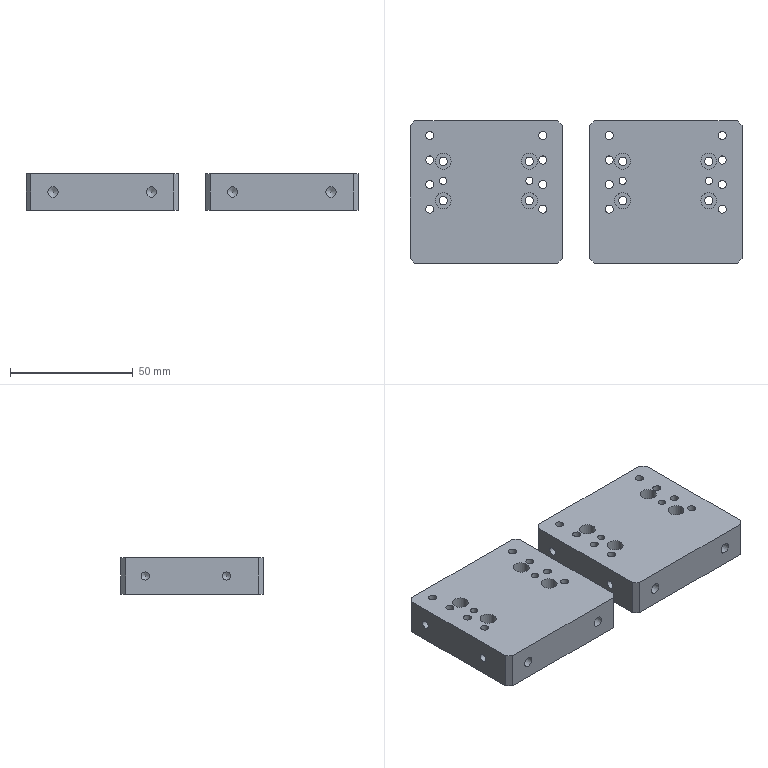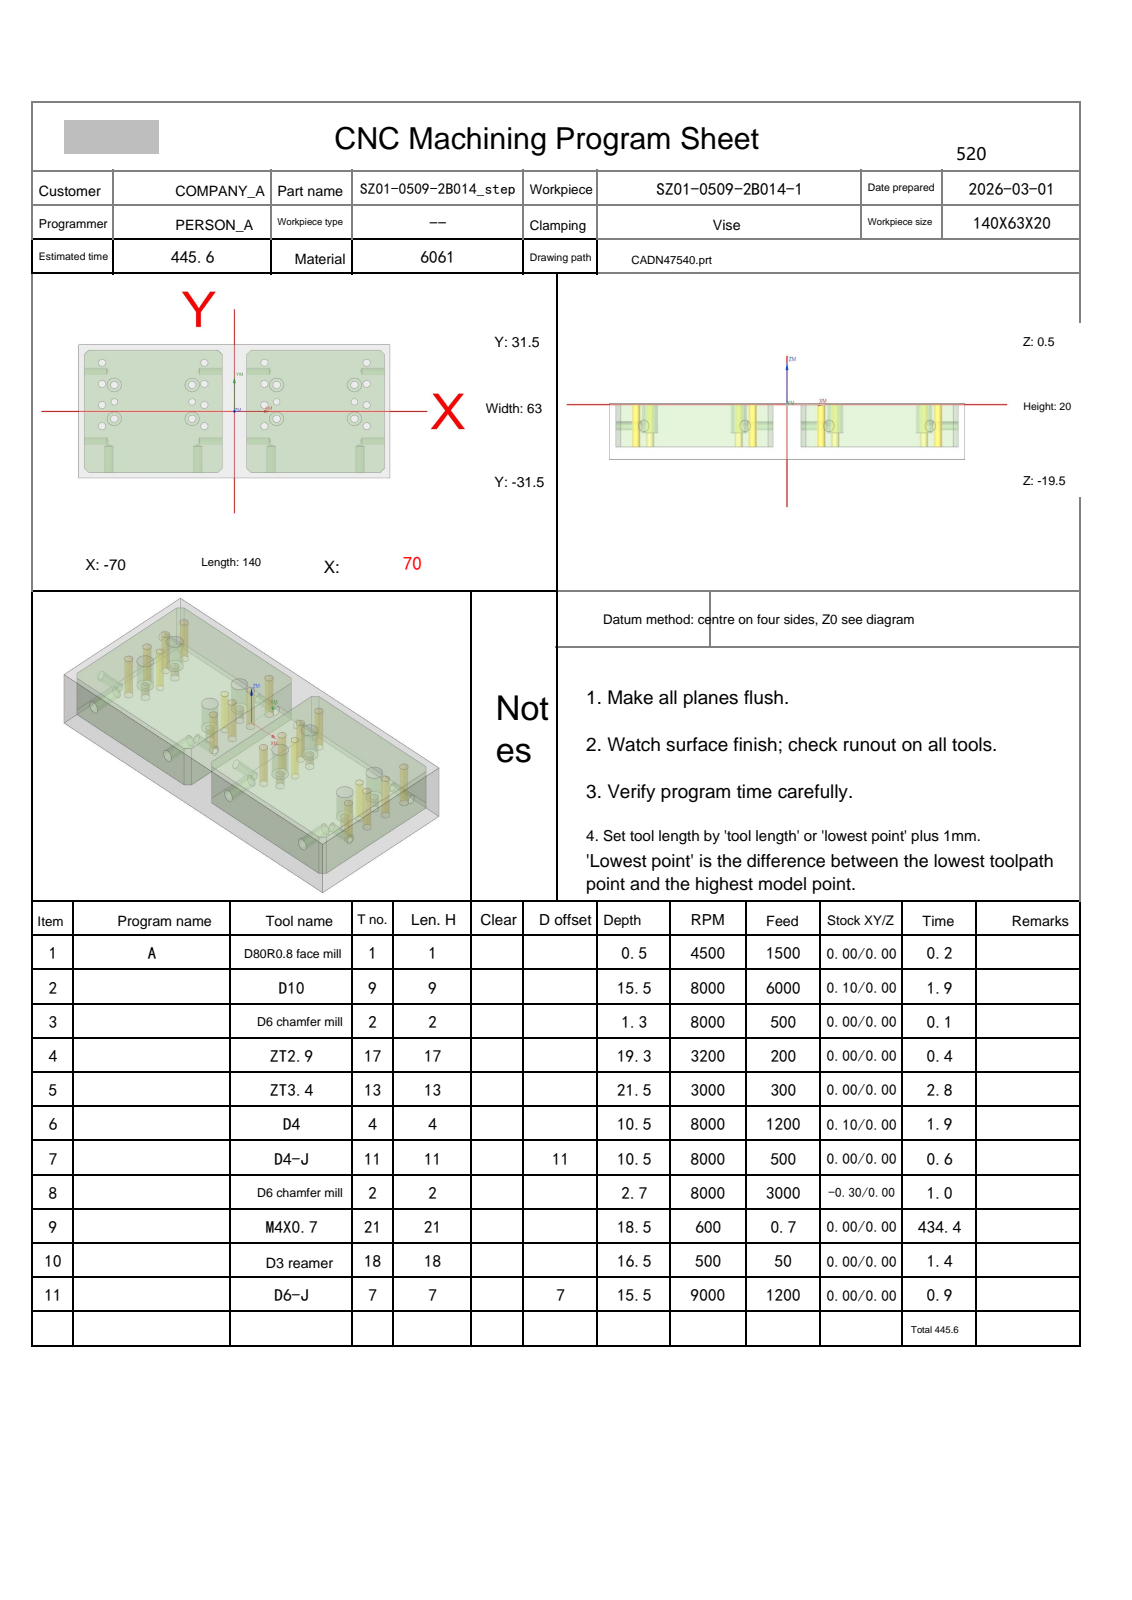NC program | NX | posted by the shop | part box 135 x 58 x 15 mm
Lines 1866 to 1983 of 1983:
N11 T07 M06
(D6-J  D=6. R=0. H=07 ce=0.00 di=0.00)
G00 G90 G54 X-6.483 Y-33.073 M03 S9000
G43 H07 Z50.
M08
Z-7.
G01 Z-7.5 F1200.
G41 D07
X-6.508 Y-32.875
G03 X-7.5 Y-32. I-.992 J-.125
G01 X-65.5
G02 X-67.621 Y-31.121 I0.0 J3.
G01 X-69.621 Y-29.121
G02 X-70.5 Y-27. I2.121 J2.121
G01 Y27.
G02 X-69.621 Y29.121 I3. J0.0
G01 X-67.621 Y31.121
G02 X-65.5 Y32. I2.121 J-2.121
G01 X-7.5
G02 X-5.379 Y31.121 I0.0 J-3.
G01 X-3.379 Y29.121
G02 X-2.5 Y27. I-2.121 J-2.121
G01 Y-27.
G02 X-3.379 Y-29.121 I-3. J0.0
G01 X-5.379 Y-31.121
G02 X-7.5 Y-32. I-2.121 J2.121
G01 X-8.
G03 X-9. Y-33. I0.0 J-1.
G01 G40 Y-33.2
Z-7.
G00 Z50.
X-6.483 Y-33.073
Z-14.5
G01 Z-15.
G41 D07
X-6.508 Y-32.875
G03 X-7.5 Y-32. I-.992 J-.125
G01 X-65.5
G02 X-67.621 Y-31.121 I0.0 J3.
G01 X-69.621 Y-29.121
G02 X-70.5 Y-27. I2.121 J2.121
G01 Y27.
G02 X-69.621 Y29.121 I3. J0.0
G01 X-67.621 Y31.121
G02 X-65.5 Y32. I2.121 J-2.121
G01 X-7.5
G02 X-5.379 Y31.121 I0.0 J-3.
G01 X-3.379 Y29.121
G02 X-2.5 Y27. I-2.121 J-2.121
G01 Y-27.
G02 X-3.379 Y-29.121 I-3. J0.0
G01 X-5.379 Y-31.121
G02 X-7.5 Y-32. I-2.121 J2.121
G01 X-8.
G03 X-9. Y-33. I0.0 J-1.
G01 G40 Y-33.2
Z-14.5
G00 Z50.
X66.517 Y-33.073
Z-7.
G01 Z-7.5
G41 D07
X66.492 Y-32.875
G03 X65.5 Y-32. I-.992 J-.125
G01 X7.5
G02 X5.379 Y-31.121 I0.0 J3.
G01 X3.379 Y-29.121
G02 X2.5 Y-27. I2.121 J2.121
G01 Y27.
G02 X3.379 Y29.121 I3. J0.0
G01 X5.379 Y31.121
G02 X7.5 Y32. I2.121 J-2.121
G01 X65.5
G02 X67.621 Y31.121 I0.0 J-3.
G01 X69.621 Y29.121
G02 X70.5 Y27. I-2.121 J-2.121
G01 Y-27.
G02 X69.621 Y-29.121 I-3. J0.0
G01 X67.621 Y-31.121
G02 X65.5 Y-32. I-2.121 J2.121
G01 X65.
G03 X64. Y-33. I0.0 J-1.
G01 G40 Y-33.2
Z-7.
G00 Z50.
X66.517 Y-33.073
Z-14.5
G01 Z-15.
G41 D07
X66.492 Y-32.875
G03 X65.5 Y-32. I-.992 J-.125
G01 X7.5
G02 X5.379 Y-31.121 I0.0 J3.
G01 X3.379 Y-29.121
G02 X2.5 Y-27. I2.121 J2.121
G01 Y27.
G02 X3.379 Y29.121 I3. J0.0
G01 X5.379 Y31.121
G02 X7.5 Y32. I2.121 J-2.121
G01 X65.5
G02 X67.621 Y31.121 I0.0 J-3.
G01 X69.621 Y29.121
G02 X70.5 Y27. I-2.121 J-2.121
G01 Y-27.
G02 X69.621 Y-29.121 I-3. J0.0
G01 X67.621 Y-31.121
G02 X65.5 Y-32. I-2.121 J2.121
G01 X65.
G03 X64. Y-33. I0.0 J-1.
G01 G40 Y-33.2
Z-14.5
G00 Z50.
M05
M09
G91 G28 Z0.0
G91 G28 Y0.0
M30
%